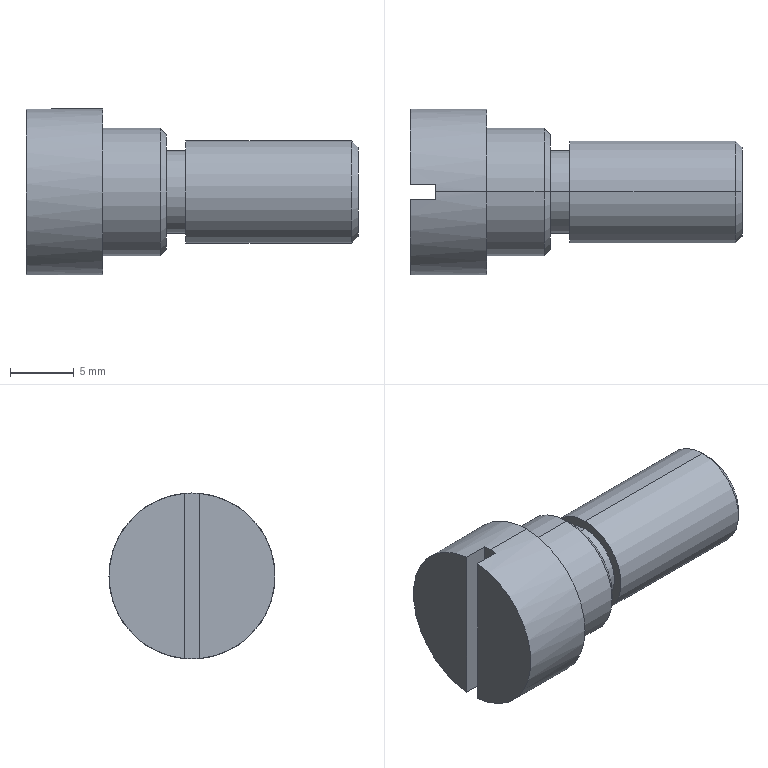Part | SolidWorks | features ICE 3, Chamfer 1, Extrusion 1, RevCut 1 | 1 solid | 21 faces | box 26 x 13 x 13 mm | volume 1879 mm3 | plane 9 | cylinder 8 | cone 4 | commonest cylinder face diameters 6.5 x2 8 x2 10 x2 13 x2
STEP:
#1=CARTESIAN_POINT('',(19.5,0.,4.));
#2=VERTEX_POINT('',#1);
#3=CARTESIAN_POINT('',(19.5,0.,-4.));
#4=VERTEX_POINT('',#3);
#5=CARTESIAN_POINT('',(19.5,0.,0.));
#6=DIRECTION('',(-1.,0.,0.));
#7=DIRECTION('',(0.,0.,-1.));
#8=AXIS2_PLACEMENT_3D('',#5,#6,#7);
#9=CIRCLE('',#8,4.);
#10=EDGE_CURVE('',#2,#4,#9,.T.);
#11=ORIENTED_EDGE('',*,*,#10,.T.);
#12=CARTESIAN_POINT('',(6.5,0.,-4.));
#13=VERTEX_POINT('',#12);
#14=CARTESIAN_POINT('',(20.,0.,-4.));
#15=DIRECTION('',(-1.,0.,0.));
#16=VECTOR('',#15,1000.);
#17=LINE('',#14,#16);
#18=EDGE_CURVE('',#4,#13,#17,.T.);
#19=ORIENTED_EDGE('',*,*,#18,.T.);
#20=CARTESIAN_POINT('',(6.5,0.,4.));
#21=VERTEX_POINT('',#20);
#22=CARTESIAN_POINT('',(6.5,0.,0.));
#23=DIRECTION('',(-1.,0.,0.));
#24=DIRECTION('',(0.,0.,1.));
#25=AXIS2_PLACEMENT_3D('',#22,#23,#24);
#26=CIRCLE('',#25,4.);
#27=EDGE_CURVE('',#21,#13,#26,.T.);
#28=ORIENTED_EDGE('',*,*,#27,.F.);
#29=CARTESIAN_POINT('',(20.,0.,4.));
#30=DIRECTION('',(-1.,0.,0.));
#31=VECTOR('',#30,1000.);
#32=LINE('',#29,#31);
#33=EDGE_CURVE('',#2,#21,#32,.T.);
#34=ORIENTED_EDGE('',*,*,#33,.F.);
#35=EDGE_LOOP('',(#11,#19,#28,#34));
#36=FACE_OUTER_BOUND('',#35,.T.);
#37=CARTESIAN_POINT('',(20.,0.,0.));
#38=DIRECTION('',(-1.,0.,0.));
#39=DIRECTION('',(0.,0.,1.));
#40=AXIS2_PLACEMENT_3D('',#37,#38,#39);
#41=CYLINDRICAL_SURFACE('',#40,4.);
#42=ADVANCED_FACE('',(#36),#41,.T.);
#43=CARTESIAN_POINT('',(20.,0.,-3.5));
#44=VERTEX_POINT('',#43);
#45=CARTESIAN_POINT('',(20.,0.,3.5));
#46=VERTEX_POINT('',#45);
#47=CARTESIAN_POINT('',(20.,0.,0.));
#48=DIRECTION('',(1.,0.,0.));
#49=DIRECTION('',(0.,0.,-1.));
#50=AXIS2_PLACEMENT_3D('',#47,#48,#49);
#51=CIRCLE('',#50,3.5);
#52=EDGE_CURVE('',#44,#46,#51,.T.);
#53=ORIENTED_EDGE('',*,*,#52,.F.);
#54=CARTESIAN_POINT('',(20.,0.,-3.5));
#55=DIRECTION('',(-0.7071,0.,-0.7071));
#56=VECTOR('',#55,1000.);
#57=LINE('',#54,#56);
#58=EDGE_CURVE('',#44,#4,#57,.T.);
#59=ORIENTED_EDGE('',*,*,#58,.T.);
#60=ORIENTED_EDGE('',*,*,#10,.F.);
#61=CARTESIAN_POINT('',(20.,0.,3.5));
#62=DIRECTION('',(-0.7071,0.,0.7071));
#63=VECTOR('',#62,1000.);
#64=LINE('',#61,#63);
#65=EDGE_CURVE('',#46,#2,#64,.T.);
#66=ORIENTED_EDGE('',*,*,#65,.F.);
#67=EDGE_LOOP('',(#53,#59,#60,#66));
#68=FACE_OUTER_BOUND('',#67,.T.);
#69=CARTESIAN_POINT('',(20.,0.,0.));
#70=DIRECTION('',(-1.,0.,0.));
#71=DIRECTION('',(0.,0.,1.));
#72=AXIS2_PLACEMENT_3D('',#69,#70,#71);
#73=CONICAL_SURFACE('',#72,3.5,0.7854);
#74=ADVANCED_FACE('',(#68),#73,.T.);
#75=CARTESIAN_POINT('',(6.5,0.,3.25));
#76=VERTEX_POINT('',#75);
#77=CARTESIAN_POINT('',(6.5,0.,-3.25));
#78=VERTEX_POINT('',#77);
#79=CARTESIAN_POINT('',(6.5,0.,0.));
#80=DIRECTION('',(-1.,0.,0.));
#81=DIRECTION('',(0.,0.,1.));
#82=AXIS2_PLACEMENT_3D('',#79,#80,#81);
#83=CIRCLE('',#82,3.25);
#84=EDGE_CURVE('',#76,#78,#83,.T.);
#85=ORIENTED_EDGE('',*,*,#84,.T.);
#86=CARTESIAN_POINT('',(5.,0.,-3.25));
#87=VERTEX_POINT('',#86);
#88=CARTESIAN_POINT('',(0.,0.,-3.25));
#89=DIRECTION('',(-1.,0.,0.));
#90=VECTOR('',#89,1000.);
#91=LINE('',#88,#90);
#92=EDGE_CURVE('',#78,#87,#91,.T.);
#93=ORIENTED_EDGE('',*,*,#92,.T.);
#94=CARTESIAN_POINT('',(5.,0.,3.25));
#95=VERTEX_POINT('',#94);
#96=CARTESIAN_POINT('',(5.,0.,0.));
#97=DIRECTION('',(-1.,0.,0.));
#98=DIRECTION('',(0.,0.,1.));
#99=AXIS2_PLACEMENT_3D('',#96,#97,#98);
#100=CIRCLE('',#99,3.25);
#101=EDGE_CURVE('',#95,#87,#100,.T.);
#102=ORIENTED_EDGE('',*,*,#101,.F.);
#103=CARTESIAN_POINT('',(0.,0.,3.25));
#104=DIRECTION('',(-1.,0.,0.));
#105=VECTOR('',#104,1000.);
#106=LINE('',#103,#105);
#107=EDGE_CURVE('',#76,#95,#106,.T.);
#108=ORIENTED_EDGE('',*,*,#107,.F.);
#109=EDGE_LOOP('',(#85,#93,#102,#108));
#110=FACE_OUTER_BOUND('',#109,.T.);
#111=CARTESIAN_POINT('',(0.,0.,0.));
#112=DIRECTION('',(-1.,0.,0.));
#113=DIRECTION('',(0.,0.,1.));
#114=AXIS2_PLACEMENT_3D('',#111,#112,#113);
#115=CYLINDRICAL_SURFACE('',#114,3.25);
#116=ADVANCED_FACE('',(#110),#115,.T.);
#117=CARTESIAN_POINT('',(5.,0.,-4.5));
#118=VERTEX_POINT('',#117);
#119=CARTESIAN_POINT('',(5.,0.,4.5));
#120=VERTEX_POINT('',#119);
#121=CARTESIAN_POINT('',(5.,0.,0.));
#122=DIRECTION('',(1.,0.,0.));
#123=DIRECTION('',(0.,0.,-1.));
#124=AXIS2_PLACEMENT_3D('',#121,#122,#123);
#125=CIRCLE('',#124,4.5);
#126=EDGE_CURVE('',#118,#120,#125,.T.);
#127=ORIENTED_EDGE('',*,*,#126,.F.);
#128=CARTESIAN_POINT('',(4.5,0.,-5.));
#129=VERTEX_POINT('',#128);
#130=CARTESIAN_POINT('',(5.,0.,-4.5));
#131=DIRECTION('',(-0.7071,0.,-0.7071));
#132=VECTOR('',#131,1000.);
#133=LINE('',#130,#132);
#134=EDGE_CURVE('',#118,#129,#133,.T.);
#135=ORIENTED_EDGE('',*,*,#134,.T.);
#136=CARTESIAN_POINT('',(4.5,0.,5.));
#137=VERTEX_POINT('',#136);
#138=CARTESIAN_POINT('',(4.5,0.,0.));
#139=DIRECTION('',(-1.,0.,0.));
#140=DIRECTION('',(0.,0.,-1.));
#141=AXIS2_PLACEMENT_3D('',#138,#139,#140);
#142=CIRCLE('',#141,5.);
#143=EDGE_CURVE('',#137,#129,#142,.T.);
#144=ORIENTED_EDGE('',*,*,#143,.F.);
#145=CARTESIAN_POINT('',(5.,0.,4.5));
#146=DIRECTION('',(-0.7071,0.,0.7071));
#147=VECTOR('',#146,1000.);
#148=LINE('',#145,#147);
#149=EDGE_CURVE('',#120,#137,#148,.T.);
#150=ORIENTED_EDGE('',*,*,#149,.F.);
#151=EDGE_LOOP('',(#127,#135,#144,#150));
#152=FACE_OUTER_BOUND('',#151,.T.);
#153=CARTESIAN_POINT('',(5.,0.,0.));
#154=DIRECTION('',(-1.,0.,0.));
#155=DIRECTION('',(0.,0.,1.));
#156=AXIS2_PLACEMENT_3D('',#153,#154,#155);
#157=CONICAL_SURFACE('',#156,4.5,0.7854);
#158=ADVANCED_FACE('',(#152),#157,.T.);
#159=CARTESIAN_POINT('',(-4.,0.,6.5));
#160=VERTEX_POINT('',#159);
#161=CARTESIAN_POINT('',(-4.,0.6,6.472));
#162=VERTEX_POINT('',#161);
#163=CARTESIAN_POINT('',(-4.,0.,0.));
#164=DIRECTION('',(-1.,0.,0.));
#165=DIRECTION('',(0.,0.,1.));
#166=AXIS2_PLACEMENT_3D('',#163,#164,#165);
#167=CIRCLE('',#166,6.5);
#168=EDGE_CURVE('',#160,#162,#167,.T.);
#169=ORIENTED_EDGE('',*,*,#168,.F.);
#170=CARTESIAN_POINT('',(0.,0.,6.5));
#171=VERTEX_POINT('',#170);
#172=CARTESIAN_POINT('',(-6.,0.,6.5));
#173=DIRECTION('',(1.,0.,0.));
#174=VECTOR('',#173,1000.);
#175=LINE('',#172,#174);
#176=EDGE_CURVE('',#160,#171,#175,.T.);
#177=ORIENTED_EDGE('',*,*,#176,.T.);
#178=CARTESIAN_POINT('',(0.,0.,-6.5));
#179=VERTEX_POINT('',#178);
#180=CARTESIAN_POINT('',(0.,0.,0.));
#181=DIRECTION('',(-1.,0.,0.));
#182=DIRECTION('',(0.,0.,1.));
#183=AXIS2_PLACEMENT_3D('',#180,#181,#182);
#184=CIRCLE('',#183,6.5);
#185=EDGE_CURVE('',#171,#179,#184,.T.);
#186=ORIENTED_EDGE('',*,*,#185,.T.);
#187=CARTESIAN_POINT('',(-4.,0.,-6.5));
#188=VERTEX_POINT('',#187);
#189=CARTESIAN_POINT('',(-6.,0.,-6.5));
#190=DIRECTION('',(1.,0.,0.));
#191=VECTOR('',#190,1000.);
#192=LINE('',#189,#191);
#193=EDGE_CURVE('',#188,#179,#192,.T.);
#194=ORIENTED_EDGE('',*,*,#193,.F.);
#195=CARTESIAN_POINT('',(-4.,0.6,-6.472));
#196=VERTEX_POINT('',#195);
#197=CARTESIAN_POINT('',(-4.,0.,0.));
#198=DIRECTION('',(-1.,0.,0.));
#199=DIRECTION('',(0.,0.,1.));
#200=AXIS2_PLACEMENT_3D('',#197,#198,#199);
#201=CIRCLE('',#200,6.5);
#202=EDGE_CURVE('',#196,#188,#201,.T.);
#203=ORIENTED_EDGE('',*,*,#202,.F.);
#204=CARTESIAN_POINT('',(-6.,0.6,-6.472));
#205=VERTEX_POINT('',#204);
#206=CARTESIAN_POINT('',(-6.,0.6,-6.472));
#207=DIRECTION('',(-1.,0.,0.));
#208=VECTOR('',#207,1000.);
#209=LINE('',#206,#208);
#210=EDGE_CURVE('',#196,#205,#209,.T.);
#211=ORIENTED_EDGE('',*,*,#210,.T.);
#212=CARTESIAN_POINT('',(-6.,0.6,6.472));
#213=VERTEX_POINT('',#212);
#214=CARTESIAN_POINT('',(-6.,0.,0.));
#215=DIRECTION('',(-1.,0.,0.));
#216=DIRECTION('',(0.,0.,1.));
#217=AXIS2_PLACEMENT_3D('',#214,#215,#216);
#218=CIRCLE('',#217,6.5);
#219=EDGE_CURVE('',#213,#205,#218,.T.);
#220=ORIENTED_EDGE('',*,*,#219,.F.);
#221=CARTESIAN_POINT('',(-6.,0.6,6.472));
#222=DIRECTION('',(1.,0.,0.));
#223=VECTOR('',#222,1000.);
#224=LINE('',#221,#223);
#225=EDGE_CURVE('',#213,#162,#224,.T.);
#226=ORIENTED_EDGE('',*,*,#225,.T.);
#227=EDGE_LOOP('',(#169,#177,#186,#194,#203,#211,#220,#226));
#228=FACE_OUTER_BOUND('',#227,.T.);
#229=CARTESIAN_POINT('',(-6.,0.,0.));
#230=DIRECTION('',(1.,0.,0.));
#231=DIRECTION('',(0.,0.,-1.));
#232=AXIS2_PLACEMENT_3D('',#229,#230,#231);
#233=CYLINDRICAL_SURFACE('',#232,6.5);
#234=ADVANCED_FACE('',(#228),#233,.T.);
#235=ORIENTED_EDGE('',*,*,#143,.T.);
#236=CARTESIAN_POINT('',(0.,0.,-5.));
#237=VERTEX_POINT('',#236);
#238=CARTESIAN_POINT('',(5.,0.,-5.));
#239=DIRECTION('',(-1.,0.,0.));
#240=VECTOR('',#239,1000.);
#241=LINE('',#238,#240);
#242=EDGE_CURVE('',#129,#237,#241,.T.);
#243=ORIENTED_EDGE('',*,*,#242,.T.);
#244=CARTESIAN_POINT('',(0.,0.,5.));
#245=VERTEX_POINT('',#244);
#246=CARTESIAN_POINT('',(0.,0.,0.));
#247=DIRECTION('',(-1.,0.,0.));
#248=DIRECTION('',(0.,0.,1.));
#249=AXIS2_PLACEMENT_3D('',#246,#247,#248);
#250=CIRCLE('',#249,5.);
#251=EDGE_CURVE('',#245,#237,#250,.T.);
#252=ORIENTED_EDGE('',*,*,#251,.F.);
#253=CARTESIAN_POINT('',(5.,0.,5.));
#254=DIRECTION('',(-1.,0.,0.));
#255=VECTOR('',#254,1000.);
#256=LINE('',#253,#255);
#257=EDGE_CURVE('',#137,#245,#256,.T.);
#258=ORIENTED_EDGE('',*,*,#257,.F.);
#259=EDGE_LOOP('',(#235,#243,#252,#258));
#260=FACE_OUTER_BOUND('',#259,.T.);
#261=CARTESIAN_POINT('',(5.,0.,0.));
#262=DIRECTION('',(-1.,0.,0.));
#263=DIRECTION('',(0.,0.,1.));
#264=AXIS2_PLACEMENT_3D('',#261,#262,#263);
#265=CYLINDRICAL_SURFACE('',#264,5.);
#266=ADVANCED_FACE('',(#260),#265,.T.);
#267=CARTESIAN_POINT('',(5.,0.,0.));
#268=DIRECTION('',(1.,0.,0.));
#269=DIRECTION('',(0.,0.,-1.));
#270=AXIS2_PLACEMENT_3D('',#267,#268,#269);
#271=CIRCLE('',#270,4.5);
#272=EDGE_CURVE('',#120,#118,#271,.T.);
#273=ORIENTED_EDGE('',*,*,#272,.T.);
#274=ORIENTED_EDGE('',*,*,#126,.T.);
#275=EDGE_LOOP('',(#273,#274));
#276=FACE_OUTER_BOUND('',#275,.T.);
#277=ORIENTED_EDGE('',*,*,#101,.T.);
#278=CARTESIAN_POINT('',(5.,0.,0.));
#279=DIRECTION('',(-1.,0.,0.));
#280=DIRECTION('',(0.,0.,1.));
#281=AXIS2_PLACEMENT_3D('',#278,#279,#280);
#282=CIRCLE('',#281,3.25);
#283=EDGE_CURVE('',#87,#95,#282,.T.);
#284=ORIENTED_EDGE('',*,*,#283,.T.);
#285=EDGE_LOOP('',(#277,#284));
#286=FACE_BOUND('',#285,.T.);
#287=CARTESIAN_POINT('',(5.,0.,0.));
#288=DIRECTION('',(1.,0.,0.));
#289=DIRECTION('',(0.,0.,-1.));
#290=AXIS2_PLACEMENT_3D('',#287,#288,#289);
#291=PLANE('',#290);
#292=ADVANCED_FACE('',(#276,#286),#291,.T.);
#293=CARTESIAN_POINT('',(-6.,-0.6,-6.472));
#294=VERTEX_POINT('',#293);
#295=CARTESIAN_POINT('',(-6.,-0.6,6.472));
#296=VERTEX_POINT('',#295);
#297=CARTESIAN_POINT('',(-6.,-0.6,0.));
#298=DIRECTION('',(0.,0.,1.));
#299=VECTOR('',#298,1000.);
#300=LINE('',#297,#299);
#301=EDGE_CURVE('',#294,#296,#300,.T.);
#302=ORIENTED_EDGE('',*,*,#301,.F.);
#303=CARTESIAN_POINT('',(-6.,0.,0.));
#304=DIRECTION('',(-1.,0.,0.));
#305=DIRECTION('',(0.,0.,1.));
#306=AXIS2_PLACEMENT_3D('',#303,#304,#305);
#307=CIRCLE('',#306,6.5);
#308=EDGE_CURVE('',#294,#296,#307,.T.);
#309=ORIENTED_EDGE('',*,*,#308,.T.);
#310=EDGE_LOOP('',(#302,#309));
#311=FACE_OUTER_BOUND('',#310,.T.);
#312=CARTESIAN_POINT('',(-6.,0.,0.));
#313=DIRECTION('',(-1.,0.,0.));
#314=DIRECTION('',(0.,0.,1.));
#315=AXIS2_PLACEMENT_3D('',#312,#313,#314);
#316=PLANE('',#315);
#317=ADVANCED_FACE('',(#311),#316,.T.);
#318=ORIENTED_EDGE('',*,*,#242,.F.);
#319=CARTESIAN_POINT('',(4.5,0.,0.));
#320=DIRECTION('',(-1.,0.,0.));
#321=DIRECTION('',(0.,0.,-1.));
#322=AXIS2_PLACEMENT_3D('',#319,#320,#321);
#323=CIRCLE('',#322,5.);
#324=EDGE_CURVE('',#129,#137,#323,.T.);
#325=ORIENTED_EDGE('',*,*,#324,.T.);
#326=ORIENTED_EDGE('',*,*,#257,.T.);
#327=CARTESIAN_POINT('',(0.,0.,0.));
#328=DIRECTION('',(-1.,0.,0.));
#329=DIRECTION('',(0.,0.,1.));
#330=AXIS2_PLACEMENT_3D('',#327,#328,#329);
#331=CIRCLE('',#330,5.);
#332=EDGE_CURVE('',#237,#245,#331,.T.);
#333=ORIENTED_EDGE('',*,*,#332,.F.);
#334=EDGE_LOOP('',(#318,#325,#326,#333));
#335=FACE_OUTER_BOUND('',#334,.T.);
#336=CARTESIAN_POINT('',(5.,0.,0.));
#337=DIRECTION('',(-1.,0.,0.));
#338=DIRECTION('',(0.,0.,1.));
#339=AXIS2_PLACEMENT_3D('',#336,#337,#338);
#340=CYLINDRICAL_SURFACE('',#339,5.);
#341=ADVANCED_FACE('',(#335),#340,.T.);
#342=CARTESIAN_POINT('',(0.,0.,0.));
#343=DIRECTION('',(-1.,0.,0.));
#344=DIRECTION('',(0.,0.,1.));
#345=AXIS2_PLACEMENT_3D('',#342,#343,#344);
#346=CIRCLE('',#345,6.5);
#347=EDGE_CURVE('',#179,#171,#346,.T.);
#348=ORIENTED_EDGE('',*,*,#347,.F.);
#349=ORIENTED_EDGE('',*,*,#185,.F.);
#350=EDGE_LOOP('',(#348,#349));
#351=FACE_OUTER_BOUND('',#350,.T.);
#352=ORIENTED_EDGE('',*,*,#251,.T.);
#353=ORIENTED_EDGE('',*,*,#332,.T.);
#354=EDGE_LOOP('',(#352,#353));
#355=FACE_BOUND('',#354,.T.);
#356=CARTESIAN_POINT('',(0.,0.,0.));
#357=DIRECTION('',(-1.,0.,0.));
#358=DIRECTION('',(0.,0.,1.));
#359=AXIS2_PLACEMENT_3D('',#356,#357,#358);
#360=PLANE('',#359);
#361=ADVANCED_FACE('',(#351,#355),#360,.F.);
#362=ORIENTED_EDGE('',*,*,#176,.F.);
#363=CARTESIAN_POINT('',(-4.,-0.6,6.472));
#364=VERTEX_POINT('',#363);
#365=CARTESIAN_POINT('',(-4.,0.,0.));
#366=DIRECTION('',(-1.,0.,0.));
#367=DIRECTION('',(0.,0.,1.));
#368=AXIS2_PLACEMENT_3D('',#365,#366,#367);
#369=CIRCLE('',#368,6.5);
#370=EDGE_CURVE('',#364,#160,#369,.T.);
#371=ORIENTED_EDGE('',*,*,#370,.F.);
#372=CARTESIAN_POINT('',(-6.,-0.6,6.472));
#373=DIRECTION('',(-1.,0.,0.));
#374=VECTOR('',#373,1000.);
#375=LINE('',#372,#374);
#376=EDGE_CURVE('',#364,#296,#375,.T.);
#377=ORIENTED_EDGE('',*,*,#376,.T.);
#378=ORIENTED_EDGE('',*,*,#308,.F.);
#379=CARTESIAN_POINT('',(-4.,-0.6,-6.472));
#380=VERTEX_POINT('',#379);
#381=CARTESIAN_POINT('',(-6.,-0.6,-6.472));
#382=DIRECTION('',(1.,0.,0.));
#383=VECTOR('',#382,1000.);
#384=LINE('',#381,#383);
#385=EDGE_CURVE('',#294,#380,#384,.T.);
#386=ORIENTED_EDGE('',*,*,#385,.T.);
#387=CARTESIAN_POINT('',(-4.,0.,0.));
#388=DIRECTION('',(-1.,0.,0.));
#389=DIRECTION('',(0.,0.,1.));
#390=AXIS2_PLACEMENT_3D('',#387,#388,#389);
#391=CIRCLE('',#390,6.5);
#392=EDGE_CURVE('',#188,#380,#391,.T.);
#393=ORIENTED_EDGE('',*,*,#392,.F.);
#394=ORIENTED_EDGE('',*,*,#193,.T.);
#395=ORIENTED_EDGE('',*,*,#347,.T.);
#396=EDGE_LOOP('',(#362,#371,#377,#378,#386,#393,#394,#395));
#397=FACE_OUTER_BOUND('',#396,.T.);
#398=CARTESIAN_POINT('',(-6.,0.,0.));
#399=DIRECTION('',(1.,0.,0.));
#400=DIRECTION('',(0.,0.,-1.));
#401=AXIS2_PLACEMENT_3D('',#398,#399,#400);
#402=CYLINDRICAL_SURFACE('',#401,6.5);
#403=ADVANCED_FACE('',(#397),#402,.T.);
#404=CARTESIAN_POINT('',(-6.,0.6,0.));
#405=DIRECTION('',(0.,0.,-1.));
#406=VECTOR('',#405,1000.);
#407=LINE('',#404,#406);
#408=EDGE_CURVE('',#213,#205,#407,.T.);
#409=ORIENTED_EDGE('',*,*,#408,.F.);
#410=ORIENTED_EDGE('',*,*,#219,.T.);
#411=EDGE_LOOP('',(#409,#410));
#412=FACE_OUTER_BOUND('',#411,.T.);
#413=CARTESIAN_POINT('',(-6.,0.,0.));
#414=DIRECTION('',(-1.,0.,0.));
#415=DIRECTION('',(0.,0.,1.));
#416=AXIS2_PLACEMENT_3D('',#413,#414,#415);
#417=PLANE('',#416);
#418=ADVANCED_FACE('',(#412),#417,.T.);
#419=ORIENTED_EDGE('',*,*,#202,.T.);
#420=ORIENTED_EDGE('',*,*,#392,.T.);
#421=CARTESIAN_POINT('',(-4.,-0.6,-15.));
#422=DIRECTION('',(0.,0.,1.));
#423=VECTOR('',#422,1000.);
#424=LINE('',#421,#423);
#425=EDGE_CURVE('',#380,#364,#424,.T.);
#426=ORIENTED_EDGE('',*,*,#425,.T.);
#427=ORIENTED_EDGE('',*,*,#370,.T.);
#428=ORIENTED_EDGE('',*,*,#168,.T.);
#429=CARTESIAN_POINT('',(-4.,0.6,-15.));
#430=DIRECTION('',(0.,0.,-1.));
#431=VECTOR('',#430,1000.);
#432=LINE('',#429,#431);
#433=EDGE_CURVE('',#162,#196,#432,.T.);
#434=ORIENTED_EDGE('',*,*,#433,.T.);
#435=EDGE_LOOP('',(#419,#420,#426,#427,#428,#434));
#436=FACE_OUTER_BOUND('',#435,.T.);
#437=CARTESIAN_POINT('',(-4.,0.,0.));
#438=DIRECTION('',(-1.,0.,0.));
#439=DIRECTION('',(0.,0.,1.));
#440=AXIS2_PLACEMENT_3D('',#437,#438,#439);
#441=PLANE('',#440);
#442=ADVANCED_FACE('',(#436),#441,.T.);
#443=ORIENTED_EDGE('',*,*,#301,.T.);
#444=ORIENTED_EDGE('',*,*,#376,.F.);
#445=ORIENTED_EDGE('',*,*,#425,.F.);
#446=ORIENTED_EDGE('',*,*,#385,.F.);
#447=EDGE_LOOP('',(#443,#444,#445,#446));
#448=FACE_OUTER_BOUND('',#447,.T.);
#449=CARTESIAN_POINT('',(-4.,-0.6,-15.));
#450=DIRECTION('',(0.,-1.,0.));
#451=DIRECTION('',(0.,0.,-1.));
#452=AXIS2_PLACEMENT_3D('',#449,#450,#451);
#453=PLANE('',#452);
#454=ADVANCED_FACE('',(#448),#453,.F.);
#455=ORIENTED_EDGE('',*,*,#408,.T.);
#456=ORIENTED_EDGE('',*,*,#210,.F.);
#457=ORIENTED_EDGE('',*,*,#433,.F.);
#458=ORIENTED_EDGE('',*,*,#225,.F.);
#459=EDGE_LOOP('',(#455,#456,#457,#458));
#460=FACE_OUTER_BOUND('',#459,.T.);
#461=CARTESIAN_POINT('',(-4.,0.6,-15.));
#462=DIRECTION('',(0.,1.,0.));
#463=DIRECTION('',(0.,0.,1.));
#464=AXIS2_PLACEMENT_3D('',#461,#462,#463);
#465=PLANE('',#464);
#466=ADVANCED_FACE('',(#460),#465,.F.);
#467=ORIENTED_EDGE('',*,*,#134,.F.);
#468=ORIENTED_EDGE('',*,*,#272,.F.);
#469=ORIENTED_EDGE('',*,*,#149,.T.);
#470=ORIENTED_EDGE('',*,*,#324,.F.);
#471=EDGE_LOOP('',(#467,#468,#469,#470));
#472=FACE_OUTER_BOUND('',#471,.T.);
#473=CARTESIAN_POINT('',(5.,0.,0.));
#474=DIRECTION('',(-1.,0.,0.));
#475=DIRECTION('',(0.,0.,1.));
#476=AXIS2_PLACEMENT_3D('',#473,#474,#475);
#477=CONICAL_SURFACE('',#476,4.5,0.7854);
#478=ADVANCED_FACE('',(#472),#477,.T.);
#479=ORIENTED_EDGE('',*,*,#84,.F.);
#480=CARTESIAN_POINT('',(6.5,0.,0.));
#481=DIRECTION('',(-1.,0.,0.));
#482=DIRECTION('',(0.,0.,1.));
#483=AXIS2_PLACEMENT_3D('',#480,#481,#482);
#484=CIRCLE('',#483,3.25);
#485=EDGE_CURVE('',#78,#76,#484,.T.);
#486=ORIENTED_EDGE('',*,*,#485,.F.);
#487=EDGE_LOOP('',(#479,#486));
#488=FACE_BOUND('',#487,.T.);
#489=ORIENTED_EDGE('',*,*,#27,.T.);
#490=CARTESIAN_POINT('',(6.5,0.,0.));
#491=DIRECTION('',(-1.,0.,0.));
#492=DIRECTION('',(0.,0.,1.));
#493=AXIS2_PLACEMENT_3D('',#490,#491,#492);
#494=CIRCLE('',#493,4.);
#495=EDGE_CURVE('',#13,#21,#494,.T.);
#496=ORIENTED_EDGE('',*,*,#495,.T.);
#497=EDGE_LOOP('',(#489,#496));
#498=FACE_OUTER_BOUND('',#497,.T.);
#499=CARTESIAN_POINT('',(6.5,0.,-3.25));
#500=DIRECTION('',(-1.,0.,0.));
#501=DIRECTION('',(0.,0.,1.));
#502=AXIS2_PLACEMENT_3D('',#499,#500,#501);
#503=PLANE('',#502);
#504=ADVANCED_FACE('',(#488,#498),#503,.T.);
#505=ORIENTED_EDGE('',*,*,#92,.F.);
#506=ORIENTED_EDGE('',*,*,#485,.T.);
#507=ORIENTED_EDGE('',*,*,#107,.T.);
#508=ORIENTED_EDGE('',*,*,#283,.F.);
#509=EDGE_LOOP('',(#505,#506,#507,#508));
#510=FACE_OUTER_BOUND('',#509,.T.);
#511=CARTESIAN_POINT('',(0.,0.,0.));
#512=DIRECTION('',(-1.,0.,0.));
#513=DIRECTION('',(0.,0.,1.));
#514=AXIS2_PLACEMENT_3D('',#511,#512,#513);
#515=CYLINDRICAL_SURFACE('',#514,3.25);
#516=ADVANCED_FACE('',(#510),#515,.T.);
#517=CARTESIAN_POINT('',(20.,0.,0.));
#518=DIRECTION('',(1.,0.,0.));
#519=DIRECTION('',(0.,0.,-1.));
#520=AXIS2_PLACEMENT_3D('',#517,#518,#519);
#521=CIRCLE('',#520,3.5);
#522=EDGE_CURVE('',#46,#44,#521,.T.);
#523=ORIENTED_EDGE('',*,*,#522,.T.);
#524=ORIENTED_EDGE('',*,*,#52,.T.);
#525=EDGE_LOOP('',(#523,#524));
#526=FACE_OUTER_BOUND('',#525,.T.);
#527=CARTESIAN_POINT('',(20.,0.,0.));
#528=DIRECTION('',(1.,0.,0.));
#529=DIRECTION('',(0.,0.,-1.));
#530=AXIS2_PLACEMENT_3D('',#527,#528,#529);
#531=PLANE('',#530);
#532=ADVANCED_FACE('',(#526),#531,.T.);
#533=ORIENTED_EDGE('',*,*,#58,.F.);
#534=ORIENTED_EDGE('',*,*,#522,.F.);
#535=ORIENTED_EDGE('',*,*,#65,.T.);
#536=CARTESIAN_POINT('',(19.5,0.,0.));
#537=DIRECTION('',(-1.,0.,0.));
#538=DIRECTION('',(0.,0.,-1.));
#539=AXIS2_PLACEMENT_3D('',#536,#537,#538);
#540=CIRCLE('',#539,4.);
#541=EDGE_CURVE('',#4,#2,#540,.T.);
#542=ORIENTED_EDGE('',*,*,#541,.F.);
#543=EDGE_LOOP('',(#533,#534,#535,#542));
#544=FACE_OUTER_BOUND('',#543,.T.);
#545=CARTESIAN_POINT('',(20.,0.,0.));
#546=DIRECTION('',(-1.,0.,0.));
#547=DIRECTION('',(0.,0.,1.));
#548=AXIS2_PLACEMENT_3D('',#545,#546,#547);
#549=CONICAL_SURFACE('',#548,3.5,0.7854);
#550=ADVANCED_FACE('',(#544),#549,.T.);
#551=ORIENTED_EDGE('',*,*,#18,.F.);
#552=ORIENTED_EDGE('',*,*,#541,.T.);
#553=ORIENTED_EDGE('',*,*,#33,.T.);
#554=ORIENTED_EDGE('',*,*,#495,.F.);
#555=EDGE_LOOP('',(#551,#552,#553,#554));
#556=FACE_OUTER_BOUND('',#555,.T.);
#557=CARTESIAN_POINT('',(20.,0.,0.));
#558=DIRECTION('',(-1.,0.,0.));
#559=DIRECTION('',(0.,0.,1.));
#560=AXIS2_PLACEMENT_3D('',#557,#558,#559);
#561=CYLINDRICAL_SURFACE('',#560,4.);
#562=ADVANCED_FACE('',(#556),#561,.T.);
#563=CLOSED_SHELL('',(#42,#74,#116,#158,#234,#266,#292,#317,#341,#361,#403,#418,#442,#454,#466,#478,#504,#516,#532,#550,#562));
#564=MANIFOLD_SOLID_BREP('',#563);
#565=CARTESIAN_POINT('',(0.,0.,0.));
#566=DIRECTION('',(0.,0.,1.));
#567=DIRECTION('',(1.,0.,0.));
#568=AXIS2_PLACEMENT_3D('',#565,#566,#567);
#569=(LENGTH_UNIT()NAMED_UNIT(*)SI_UNIT(.MILLI.,.METRE.));
#570=UNCERTAINTY_MEASURE_WITH_UNIT(LENGTH_MEASURE(0.00001),#569,'','');
#571=(NAMED_UNIT(*)PLANE_ANGLE_UNIT()SI_UNIT($,.RADIAN.));
#572=(NAMED_UNIT(*)SI_UNIT($,.STERADIAN.)SOLID_ANGLE_UNIT());
#573=(GEOMETRIC_REPRESENTATION_CONTEXT(3)GLOBAL_UNCERTAINTY_ASSIGNED_CONTEXT((#570))GLOBAL_UNIT_ASSIGNED_CONTEXT((#569,#571,#572))REPRESENTATION_CONTEXT('',''));
#574=ADVANCED_BREP_SHAPE_REPRESENTATION('',(#564,#568),#573);